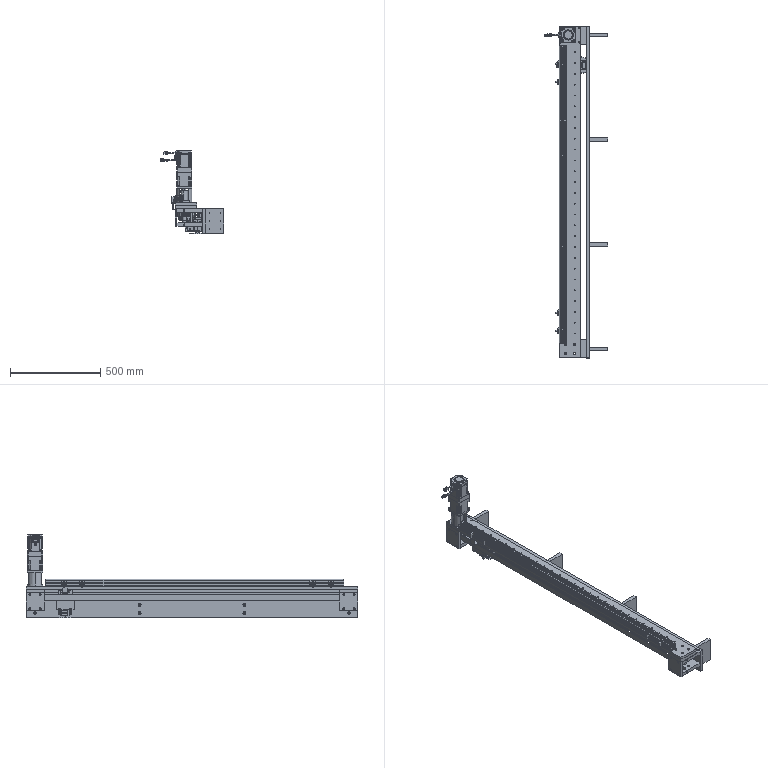Part | SolidWorks | features ReferencePattern 9, LocalLPattern 3, CompositeCurve 2 | 61 solids | 3913 faces | volume 14966347 mm3 | cylinder 1713 | plane 1705 | cone 369 | spline 126 | commonest cylinder face diameters 1 x158 5 x107 1.2 x100 9 x78 4.2 x76 6.8 x76